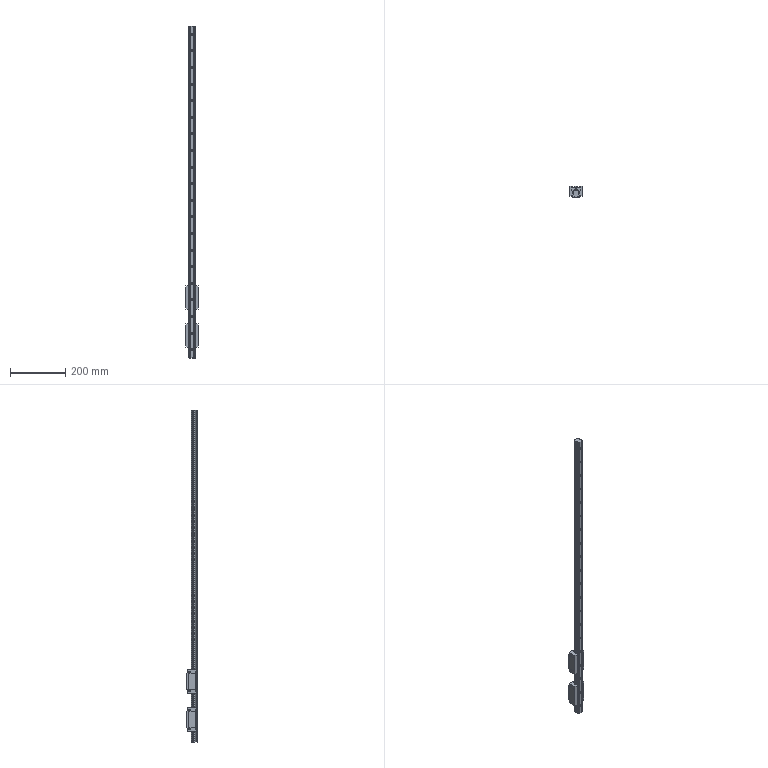Part | SolidWorks | 3 solids | 390 faces | box 48 x 40 x 1200 mm | volume 702488 mm3 | plane 206 | cylinder 168 | cone 16 | commonest cylinder face diameters 7 x40 11 x40 6 x24 1 x16 5 x16 4.6 x12